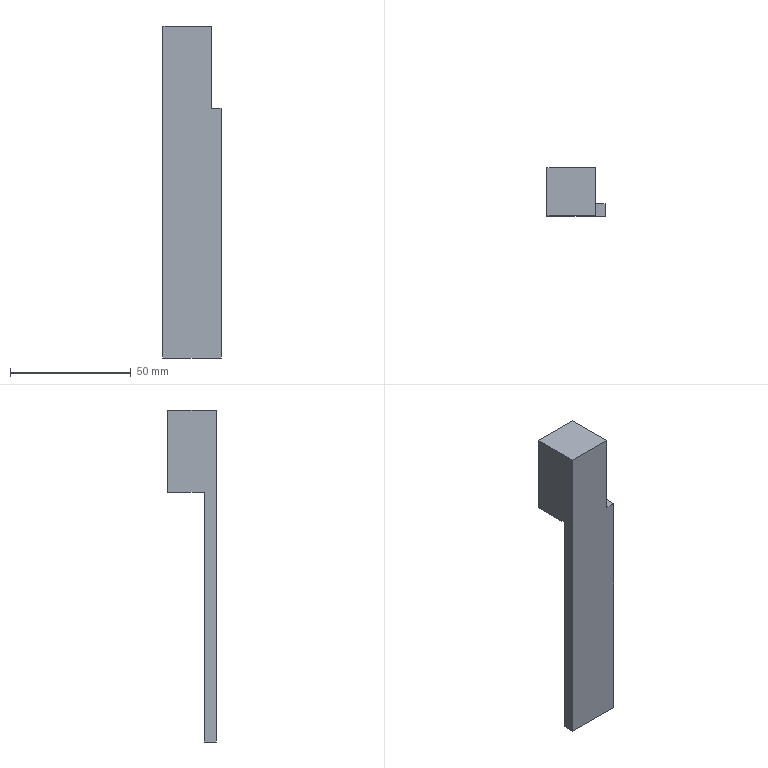Part | SolidWorks | features BaseBody 1 | 1 solid | 14 faces | box 24 x 20 x 137.345 mm | volume 25628 mm3 | plane 14
STEP:
#1=CARTESIAN_POINT('',(-7.753,369.5,-102.));
#2=VERTEX_POINT('',#1);
#3=CARTESIAN_POINT('',(-27.753,369.5,-102.));
#4=VERTEX_POINT('',#3);
#5=CARTESIAN_POINT('',(37.247,369.5,-102.));
#6=DIRECTION('',(-1.,0.,0.));
#7=VECTOR('',#6,1000.);
#8=LINE('',#5,#7);
#9=EDGE_CURVE('',#2,#4,#8,.T.);
#10=ORIENTED_EDGE('',*,*,#9,.T.);
#11=CARTESIAN_POINT('',(-27.753,369.5,-239.345));
#12=VERTEX_POINT('',#11);
#13=CARTESIAN_POINT('',(-27.753,369.5,-176.043));
#14=DIRECTION('',(0.,0.,-1.));
#15=VECTOR('',#14,1000.);
#16=LINE('',#13,#15);
#17=EDGE_CURVE('',#4,#12,#16,.T.);
#18=ORIENTED_EDGE('',*,*,#17,.T.);
#19=CARTESIAN_POINT('',(-3.753,369.5,-239.345));
#20=VERTEX_POINT('',#19);
#21=CARTESIAN_POINT('',(37.247,369.5,-239.345));
#22=DIRECTION('',(1.,0.,0.));
#23=VECTOR('',#22,1000.);
#24=LINE('',#21,#23);
#25=EDGE_CURVE('',#12,#20,#24,.T.);
#26=ORIENTED_EDGE('',*,*,#25,.T.);
#27=CARTESIAN_POINT('',(-3.753,369.5,-136.));
#28=VERTEX_POINT('',#27);
#29=CARTESIAN_POINT('',(-3.753,369.5,-176.043));
#30=DIRECTION('',(0.,0.,1.));
#31=VECTOR('',#30,1000.);
#32=LINE('',#29,#31);
#33=EDGE_CURVE('',#20,#28,#32,.T.);
#34=ORIENTED_EDGE('',*,*,#33,.T.);
#35=CARTESIAN_POINT('',(-7.753,369.5,-136.));
#36=VERTEX_POINT('',#35);
#37=CARTESIAN_POINT('',(37.247,369.5,-136.));
#38=DIRECTION('',(-1.,0.,0.));
#39=VECTOR('',#38,1000.);
#40=LINE('',#37,#39);
#41=EDGE_CURVE('',#28,#36,#40,.T.);
#42=ORIENTED_EDGE('',*,*,#41,.T.);
#43=CARTESIAN_POINT('',(-7.753,369.5,-176.043));
#44=DIRECTION('',(0.,0.,1.));
#45=VECTOR('',#44,1000.);
#46=LINE('',#43,#45);
#47=EDGE_CURVE('',#36,#2,#46,.T.);
#48=ORIENTED_EDGE('',*,*,#47,.T.);
#49=EDGE_LOOP('',(#10,#18,#26,#34,#42,#48));
#50=FACE_OUTER_BOUND('',#49,.T.);
#51=CARTESIAN_POINT('',(37.247,369.5,-176.043));
#52=DIRECTION('',(0.,-1.,0.));
#53=DIRECTION('',(0.,0.,-1.));
#54=AXIS2_PLACEMENT_3D('',#51,#52,#53);
#55=PLANE('',#54);
#56=ADVANCED_FACE('',(#50),#55,.T.);
#57=CARTESIAN_POINT('',(-27.753,389.5,-102.));
#58=VERTEX_POINT('',#57);
#59=CARTESIAN_POINT('',(-27.753,382.,-102.));
#60=DIRECTION('',(0.,1.,0.));
#61=VECTOR('',#60,1000.);
#62=LINE('',#59,#61);
#63=EDGE_CURVE('',#4,#58,#62,.T.);
#64=ORIENTED_EDGE('',*,*,#63,.T.);
#65=CARTESIAN_POINT('',(-27.753,389.5,-136.));
#66=VERTEX_POINT('',#65);
#67=CARTESIAN_POINT('',(-27.753,389.5,-176.043));
#68=DIRECTION('',(0.,0.,-1.));
#69=VECTOR('',#68,1000.);
#70=LINE('',#67,#69);
#71=EDGE_CURVE('',#58,#66,#70,.T.);
#72=ORIENTED_EDGE('',*,*,#71,.T.);
#73=CARTESIAN_POINT('',(-27.753,374.5,-136.));
#74=VERTEX_POINT('',#73);
#75=CARTESIAN_POINT('',(-27.753,382.,-136.));
#76=DIRECTION('',(0.,-1.,0.));
#77=VECTOR('',#76,1000.);
#78=LINE('',#75,#77);
#79=EDGE_CURVE('',#66,#74,#78,.T.);
#80=ORIENTED_EDGE('',*,*,#79,.T.);
#81=CARTESIAN_POINT('',(-27.753,374.5,-239.345));
#82=VERTEX_POINT('',#81);
#83=CARTESIAN_POINT('',(-27.753,374.5,-176.043));
#84=DIRECTION('',(0.,0.,-1.));
#85=VECTOR('',#84,1000.);
#86=LINE('',#83,#85);
#87=EDGE_CURVE('',#74,#82,#86,.T.);
#88=ORIENTED_EDGE('',*,*,#87,.T.);
#89=CARTESIAN_POINT('',(-27.753,382.,-239.345));
#90=DIRECTION('',(0.,-1.,0.));
#91=VECTOR('',#90,1000.);
#92=LINE('',#89,#91);
#93=EDGE_CURVE('',#82,#12,#92,.T.);
#94=ORIENTED_EDGE('',*,*,#93,.T.);
#95=ORIENTED_EDGE('',*,*,#17,.F.);
#96=EDGE_LOOP('',(#64,#72,#80,#88,#94,#95));
#97=FACE_OUTER_BOUND('',#96,.T.);
#98=CARTESIAN_POINT('',(-27.753,382.,-176.043));
#99=DIRECTION('',(-1.,0.,0.));
#100=DIRECTION('',(0.,0.,1.));
#101=AXIS2_PLACEMENT_3D('',#98,#99,#100);
#102=PLANE('',#101);
#103=ADVANCED_FACE('',(#97),#102,.T.);
#104=ORIENTED_EDGE('',*,*,#63,.F.);
#105=ORIENTED_EDGE('',*,*,#9,.F.);
#106=CARTESIAN_POINT('',(-7.753,389.5,-102.));
#107=VERTEX_POINT('',#106);
#108=CARTESIAN_POINT('',(-7.753,389.115,-102.));
#109=DIRECTION('',(0.,1.,0.));
#110=VECTOR('',#109,1000.);
#111=LINE('',#108,#110);
#112=EDGE_CURVE('',#2,#107,#111,.T.);
#113=ORIENTED_EDGE('',*,*,#112,.T.);
#114=CARTESIAN_POINT('',(-16.984,389.5,-102.));
#115=DIRECTION('',(-1.,0.,0.));
#116=VECTOR('',#115,1000.);
#117=LINE('',#114,#116);
#118=EDGE_CURVE('',#107,#58,#117,.T.);
#119=ORIENTED_EDGE('',*,*,#118,.T.);
#120=EDGE_LOOP('',(#104,#105,#113,#119));
#121=FACE_OUTER_BOUND('',#120,.T.);
#122=CARTESIAN_POINT('',(-16.984,389.115,-102.));
#123=DIRECTION('',(0.,0.,1.));
#124=DIRECTION('',(1.,0.,0.));
#125=AXIS2_PLACEMENT_3D('',#122,#123,#124);
#126=PLANE('',#125);
#127=ADVANCED_FACE('',(#121),#126,.T.);
#128=CARTESIAN_POINT('',(-7.753,389.5,-136.));
#129=VERTEX_POINT('',#128);
#130=CARTESIAN_POINT('',(-7.753,389.5,-176.043));
#131=DIRECTION('',(0.,0.,-1.));
#132=VECTOR('',#131,1000.);
#133=LINE('',#130,#132);
#134=EDGE_CURVE('',#107,#129,#133,.T.);
#135=ORIENTED_EDGE('',*,*,#134,.F.);
#136=ORIENTED_EDGE('',*,*,#112,.F.);
#137=ORIENTED_EDGE('',*,*,#47,.F.);
#138=CARTESIAN_POINT('',(-7.753,374.5,-136.));
#139=VERTEX_POINT('',#138);
#140=CARTESIAN_POINT('',(-7.753,382.,-136.));
#141=DIRECTION('',(0.,-1.,0.));
#142=VECTOR('',#141,1000.);
#143=LINE('',#140,#142);
#144=EDGE_CURVE('',#139,#36,#143,.T.);
#145=ORIENTED_EDGE('',*,*,#144,.F.);
#146=CARTESIAN_POINT('',(-7.753,382.,-136.));
#147=DIRECTION('',(0.,-1.,0.));
#148=VECTOR('',#147,1000.);
#149=LINE('',#146,#148);
#150=EDGE_CURVE('',#129,#139,#149,.T.);
#151=ORIENTED_EDGE('',*,*,#150,.F.);
#152=EDGE_LOOP('',(#135,#136,#137,#145,#151));
#153=FACE_OUTER_BOUND('',#152,.T.);
#154=CARTESIAN_POINT('',(-7.753,382.,-176.043));
#155=DIRECTION('',(-1.,0.,0.));
#156=DIRECTION('',(0.,0.,1.));
#157=AXIS2_PLACEMENT_3D('',#154,#155,#156);
#158=PLANE('',#157);
#159=ADVANCED_FACE('',(#153),#158,.F.);
#160=CARTESIAN_POINT('',(-3.753,374.5,-136.));
#161=VERTEX_POINT('',#160);
#162=CARTESIAN_POINT('',(-3.753,379.5,-136.));
#163=DIRECTION('',(0.,-1.,0.));
#164=VECTOR('',#163,1000.);
#165=LINE('',#162,#164);
#166=EDGE_CURVE('',#161,#28,#165,.T.);
#167=ORIENTED_EDGE('',*,*,#166,.F.);
#168=CARTESIAN_POINT('',(44.687,374.5,-136.));
#169=DIRECTION('',(1.,0.,0.));
#170=VECTOR('',#169,1000.);
#171=LINE('',#168,#170);
#172=EDGE_CURVE('',#139,#161,#171,.T.);
#173=ORIENTED_EDGE('',*,*,#172,.F.);
#174=ORIENTED_EDGE('',*,*,#144,.T.);
#175=ORIENTED_EDGE('',*,*,#41,.F.);
#176=EDGE_LOOP('',(#167,#173,#174,#175));
#177=FACE_OUTER_BOUND('',#176,.T.);
#178=CARTESIAN_POINT('',(44.687,379.5,-136.));
#179=DIRECTION('',(0.,0.,-1.));
#180=DIRECTION('',(-1.,0.,0.));
#181=AXIS2_PLACEMENT_3D('',#178,#179,#180);
#182=PLANE('',#181);
#183=ADVANCED_FACE('',(#177),#182,.F.);
#184=CARTESIAN_POINT('',(-3.753,372.5,-146.043));
#185=VERTEX_POINT('',#184);
#186=CARTESIAN_POINT('',(-3.753,371.5,-146.043));
#187=VERTEX_POINT('',#186);
#188=CARTESIAN_POINT('',(-3.753,382.,-146.043));
#189=DIRECTION('',(0.,-1.,0.));
#190=VECTOR('',#189,1000.);
#191=LINE('',#188,#190);
#192=EDGE_CURVE('',#185,#187,#191,.T.);
#193=ORIENTED_EDGE('',*,*,#192,.F.);
#194=CARTESIAN_POINT('',(-3.753,372.5,-239.345));
#195=VERTEX_POINT('',#194);
#196=CARTESIAN_POINT('',(-3.753,372.5,-176.043));
#197=DIRECTION('',(0.,0.,1.));
#198=VECTOR('',#197,1000.);
#199=LINE('',#196,#198);
#200=EDGE_CURVE('',#195,#185,#199,.T.);
#201=ORIENTED_EDGE('',*,*,#200,.F.);
#202=CARTESIAN_POINT('',(-3.753,374.5,-239.345));
#203=VERTEX_POINT('',#202);
#204=CARTESIAN_POINT('',(-3.753,382.,-239.345));
#205=DIRECTION('',(0.,-1.,0.));
#206=VECTOR('',#205,1000.);
#207=LINE('',#204,#206);
#208=EDGE_CURVE('',#203,#195,#207,.T.);
#209=ORIENTED_EDGE('',*,*,#208,.F.);
#210=CARTESIAN_POINT('',(-3.753,374.5,-176.043));
#211=DIRECTION('',(0.,0.,-1.));
#212=VECTOR('',#211,1000.);
#213=LINE('',#210,#212);
#214=EDGE_CURVE('',#161,#203,#213,.T.);
#215=ORIENTED_EDGE('',*,*,#214,.F.);
#216=ORIENTED_EDGE('',*,*,#166,.T.);
#217=ORIENTED_EDGE('',*,*,#33,.F.);
#218=CARTESIAN_POINT('',(-3.753,371.5,-239.345));
#219=VERTEX_POINT('',#218);
#220=CARTESIAN_POINT('',(-3.753,382.,-239.345));
#221=DIRECTION('',(0.,-1.,0.));
#222=VECTOR('',#221,1000.);
#223=LINE('',#220,#222);
#224=EDGE_CURVE('',#219,#20,#223,.T.);
#225=ORIENTED_EDGE('',*,*,#224,.F.);
#226=CARTESIAN_POINT('',(-3.753,371.5,-176.043));
#227=DIRECTION('',(0.,0.,-1.));
#228=VECTOR('',#227,1000.);
#229=LINE('',#226,#228);
#230=EDGE_CURVE('',#187,#219,#229,.T.);
#231=ORIENTED_EDGE('',*,*,#230,.F.);
#232=EDGE_LOOP('',(#193,#201,#209,#215,#216,#217,#225,#231));
#233=FACE_OUTER_BOUND('',#232,.T.);
#234=CARTESIAN_POINT('',(-3.753,382.,-176.043));
#235=DIRECTION('',(-1.,0.,0.));
#236=DIRECTION('',(0.,0.,1.));
#237=AXIS2_PLACEMENT_3D('',#234,#235,#236);
#238=PLANE('',#237);
#239=ADVANCED_FACE('',(#233),#238,.F.);
#240=CARTESIAN_POINT('',(-7.753,372.5,-239.345));
#241=VERTEX_POINT('',#240);
#242=CARTESIAN_POINT('',(-7.753,371.5,-239.345));
#243=VERTEX_POINT('',#242);
#244=CARTESIAN_POINT('',(-7.753,564.,-239.345));
#245=DIRECTION('',(0.,-1.,0.));
#246=VECTOR('',#245,1000.);
#247=LINE('',#244,#246);
#248=EDGE_CURVE('',#241,#243,#247,.T.);
#249=ORIENTED_EDGE('',*,*,#248,.T.);
#250=CARTESIAN_POINT('',(232.247,371.5,-239.345));
#251=DIRECTION('',(1.,0.,0.));
#252=VECTOR('',#251,1000.);
#253=LINE('',#250,#252);
#254=EDGE_CURVE('',#243,#219,#253,.T.);
#255=ORIENTED_EDGE('',*,*,#254,.T.);
#256=ORIENTED_EDGE('',*,*,#224,.T.);
#257=ORIENTED_EDGE('',*,*,#25,.F.);
#258=ORIENTED_EDGE('',*,*,#93,.F.);
#259=CARTESIAN_POINT('',(232.247,374.5,-239.345));
#260=DIRECTION('',(1.,0.,0.));
#261=VECTOR('',#260,1000.);
#262=LINE('',#259,#261);
#263=EDGE_CURVE('',#82,#203,#262,.T.);
#264=ORIENTED_EDGE('',*,*,#263,.T.);
#265=ORIENTED_EDGE('',*,*,#208,.T.);
#266=CARTESIAN_POINT('',(232.247,372.5,-239.345));
#267=DIRECTION('',(-1.,0.,0.));
#268=VECTOR('',#267,1000.);
#269=LINE('',#266,#268);
#270=EDGE_CURVE('',#195,#241,#269,.T.);
#271=ORIENTED_EDGE('',*,*,#270,.T.);
#272=EDGE_LOOP('',(#249,#255,#256,#257,#258,#264,#265,#271));
#273=FACE_OUTER_BOUND('',#272,.T.);
#274=CARTESIAN_POINT('',(232.247,564.,-239.345));
#275=DIRECTION('',(0.,0.,-1.));
#276=DIRECTION('',(-1.,0.,0.));
#277=AXIS2_PLACEMENT_3D('',#274,#275,#276);
#278=PLANE('',#277);
#279=ADVANCED_FACE('',(#273),#278,.T.);
#280=ORIENTED_EDGE('',*,*,#118,.F.);
#281=ORIENTED_EDGE('',*,*,#134,.T.);
#282=CARTESIAN_POINT('',(62.862,389.5,-136.));
#283=DIRECTION('',(-1.,0.,0.));
#284=VECTOR('',#283,1000.);
#285=LINE('',#282,#284);
#286=EDGE_CURVE('',#129,#66,#285,.T.);
#287=ORIENTED_EDGE('',*,*,#286,.T.);
#288=ORIENTED_EDGE('',*,*,#71,.F.);
#289=EDGE_LOOP('',(#280,#281,#287,#288));
#290=FACE_OUTER_BOUND('',#289,.T.);
#291=CARTESIAN_POINT('',(62.862,389.5,-444.615));
#292=DIRECTION('',(0.,1.,0.));
#293=DIRECTION('',(0.,0.,1.));
#294=AXIS2_PLACEMENT_3D('',#291,#292,#293);
#295=PLANE('',#294);
#296=ADVANCED_FACE('',(#290),#295,.T.);
#297=ORIENTED_EDGE('',*,*,#214,.T.);
#298=ORIENTED_EDGE('',*,*,#263,.F.);
#299=ORIENTED_EDGE('',*,*,#87,.F.);
#300=CARTESIAN_POINT('',(357.247,374.5,-136.));
#301=DIRECTION('',(-1.,0.,0.));
#302=VECTOR('',#301,1000.);
#303=LINE('',#300,#302);
#304=EDGE_CURVE('',#139,#74,#303,.T.);
#305=ORIENTED_EDGE('',*,*,#304,.F.);
#306=ORIENTED_EDGE('',*,*,#172,.T.);
#307=EDGE_LOOP('',(#297,#298,#299,#305,#306));
#308=FACE_OUTER_BOUND('',#307,.T.);
#309=CARTESIAN_POINT('',(357.247,374.5,-344.345));
#310=DIRECTION('',(0.,-1.,0.));
#311=DIRECTION('',(0.,0.,-1.));
#312=AXIS2_PLACEMENT_3D('',#309,#310,#311);
#313=PLANE('',#312);
#314=ADVANCED_FACE('',(#308),#313,.F.);
#315=ORIENTED_EDGE('',*,*,#150,.T.);
#316=ORIENTED_EDGE('',*,*,#304,.T.);
#317=ORIENTED_EDGE('',*,*,#79,.F.);
#318=ORIENTED_EDGE('',*,*,#286,.F.);
#319=EDGE_LOOP('',(#315,#316,#317,#318));
#320=FACE_OUTER_BOUND('',#319,.T.);
#321=CARTESIAN_POINT('',(44.687,379.5,-136.));
#322=DIRECTION('',(0.,0.,-1.));
#323=DIRECTION('',(-1.,0.,0.));
#324=AXIS2_PLACEMENT_3D('',#321,#322,#323);
#325=PLANE('',#324);
#326=ADVANCED_FACE('',(#320),#325,.T.);
#327=CARTESIAN_POINT('',(-7.753,371.5,-146.043));
#328=VERTEX_POINT('',#327);
#329=CARTESIAN_POINT('',(57.247,371.5,-146.043));
#330=DIRECTION('',(-1.,0.,0.));
#331=VECTOR('',#330,1000.);
#332=LINE('',#329,#331);
#333=EDGE_CURVE('',#187,#328,#332,.T.);
#334=ORIENTED_EDGE('',*,*,#333,.F.);
#335=ORIENTED_EDGE('',*,*,#230,.T.);
#336=ORIENTED_EDGE('',*,*,#254,.F.);
#337=CARTESIAN_POINT('',(-7.753,371.5,-276.043));
#338=DIRECTION('',(0.,0.,-1.));
#339=VECTOR('',#338,1000.);
#340=LINE('',#337,#339);
#341=EDGE_CURVE('',#328,#243,#340,.T.);
#342=ORIENTED_EDGE('',*,*,#341,.F.);
#343=EDGE_LOOP('',(#334,#335,#336,#342));
#344=FACE_OUTER_BOUND('',#343,.T.);
#345=CARTESIAN_POINT('',(57.247,371.5,-276.043));
#346=DIRECTION('',(0.,-1.,0.));
#347=DIRECTION('',(0.,0.,-1.));
#348=AXIS2_PLACEMENT_3D('',#345,#346,#347);
#349=PLANE('',#348);
#350=ADVANCED_FACE('',(#344),#349,.F.);
#351=CARTESIAN_POINT('',(-7.753,372.5,-146.043));
#352=VERTEX_POINT('',#351);
#353=CARTESIAN_POINT('',(57.247,372.5,-146.043));
#354=DIRECTION('',(-1.,0.,0.));
#355=VECTOR('',#354,1000.);
#356=LINE('',#353,#355);
#357=EDGE_CURVE('',#185,#352,#356,.T.);
#358=ORIENTED_EDGE('',*,*,#357,.F.);
#359=ORIENTED_EDGE('',*,*,#192,.T.);
#360=ORIENTED_EDGE('',*,*,#333,.T.);
#361=CARTESIAN_POINT('',(-7.753,372.,-146.043));
#362=DIRECTION('',(0.,-1.,0.));
#363=VECTOR('',#362,1000.);
#364=LINE('',#361,#363);
#365=EDGE_CURVE('',#352,#328,#364,.T.);
#366=ORIENTED_EDGE('',*,*,#365,.F.);
#367=EDGE_LOOP('',(#358,#359,#360,#366));
#368=FACE_OUTER_BOUND('',#367,.T.);
#369=CARTESIAN_POINT('',(57.247,372.,-146.043));
#370=DIRECTION('',(0.,0.,1.));
#371=DIRECTION('',(1.,0.,0.));
#372=AXIS2_PLACEMENT_3D('',#369,#370,#371);
#373=PLANE('',#372);
#374=ADVANCED_FACE('',(#368),#373,.F.);
#375=ORIENTED_EDGE('',*,*,#357,.T.);
#376=CARTESIAN_POINT('',(-7.753,372.5,-276.043));
#377=DIRECTION('',(0.,0.,1.));
#378=VECTOR('',#377,1000.);
#379=LINE('',#376,#378);
#380=EDGE_CURVE('',#241,#352,#379,.T.);
#381=ORIENTED_EDGE('',*,*,#380,.F.);
#382=ORIENTED_EDGE('',*,*,#270,.F.);
#383=ORIENTED_EDGE('',*,*,#200,.T.);
#384=EDGE_LOOP('',(#375,#381,#382,#383));
#385=FACE_OUTER_BOUND('',#384,.T.);
#386=CARTESIAN_POINT('',(57.247,372.5,-276.043));
#387=DIRECTION('',(0.,1.,0.));
#388=DIRECTION('',(0.,0.,1.));
#389=AXIS2_PLACEMENT_3D('',#386,#387,#388);
#390=PLANE('',#389);
#391=ADVANCED_FACE('',(#385),#390,.F.);
#392=ORIENTED_EDGE('',*,*,#365,.T.);
#393=ORIENTED_EDGE('',*,*,#341,.T.);
#394=ORIENTED_EDGE('',*,*,#248,.F.);
#395=ORIENTED_EDGE('',*,*,#380,.T.);
#396=EDGE_LOOP('',(#392,#393,#394,#395));
#397=FACE_OUTER_BOUND('',#396,.T.);
#398=CARTESIAN_POINT('',(-7.753,372.,-276.043));
#399=DIRECTION('',(-1.,0.,0.));
#400=DIRECTION('',(0.,0.,1.));
#401=AXIS2_PLACEMENT_3D('',#398,#399,#400);
#402=PLANE('',#401);
#403=ADVANCED_FACE('',(#397),#402,.F.);
#404=CLOSED_SHELL('',(#56,#103,#127,#159,#183,#239,#279,#296,#314,#326,#350,#374,#391,#403));
#405=MANIFOLD_SOLID_BREP('',#404);
#406=CARTESIAN_POINT('',(0.,0.,0.));
#407=DIRECTION('',(0.,0.,1.));
#408=DIRECTION('',(1.,0.,0.));
#409=AXIS2_PLACEMENT_3D('',#406,#407,#408);
#410=(LENGTH_UNIT()NAMED_UNIT(*)SI_UNIT(.MILLI.,.METRE.));
#411=UNCERTAINTY_MEASURE_WITH_UNIT(LENGTH_MEASURE(0.00001),#410,'','');
#412=(NAMED_UNIT(*)PLANE_ANGLE_UNIT()SI_UNIT($,.RADIAN.));
#413=(NAMED_UNIT(*)SI_UNIT($,.STERADIAN.)SOLID_ANGLE_UNIT());
#414=(GEOMETRIC_REPRESENTATION_CONTEXT(3)GLOBAL_UNCERTAINTY_ASSIGNED_CONTEXT((#411))GLOBAL_UNIT_ASSIGNED_CONTEXT((#410,#412,#413))REPRESENTATION_CONTEXT('',''));
#415=ADVANCED_BREP_SHAPE_REPRESENTATION('',(#405,#409),#414);